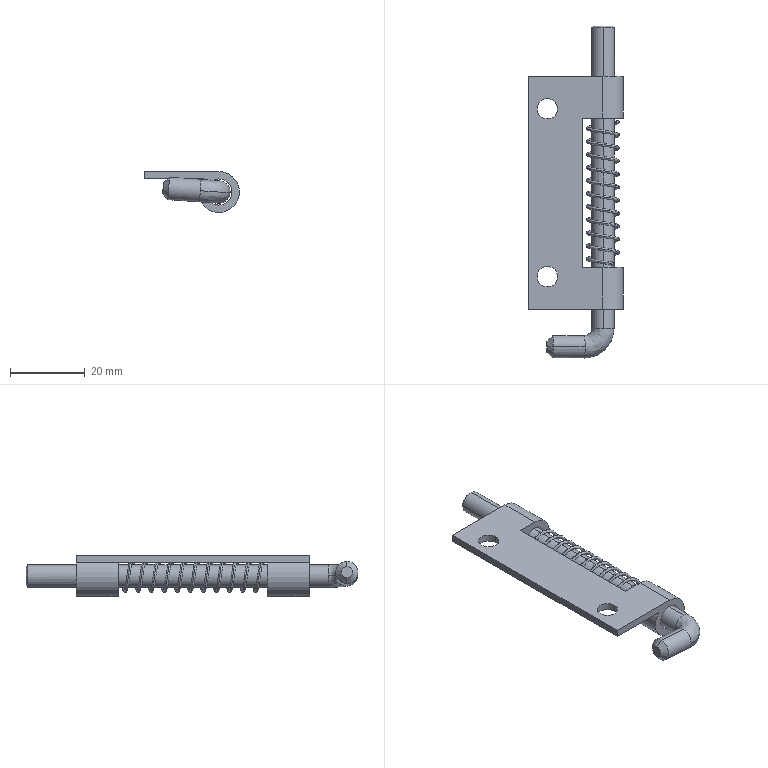Part | SolidWorks | features MirrorStock 1 | 3 solids | 38 faces | box 25.4 x 89 x 11 mm | volume 6004 mm3 | cylinder 14 | plane 12 | spline 8 | cone 4 | commonest cylinder face diameters 5.5 x4 6 x4 7 x4 11 x2